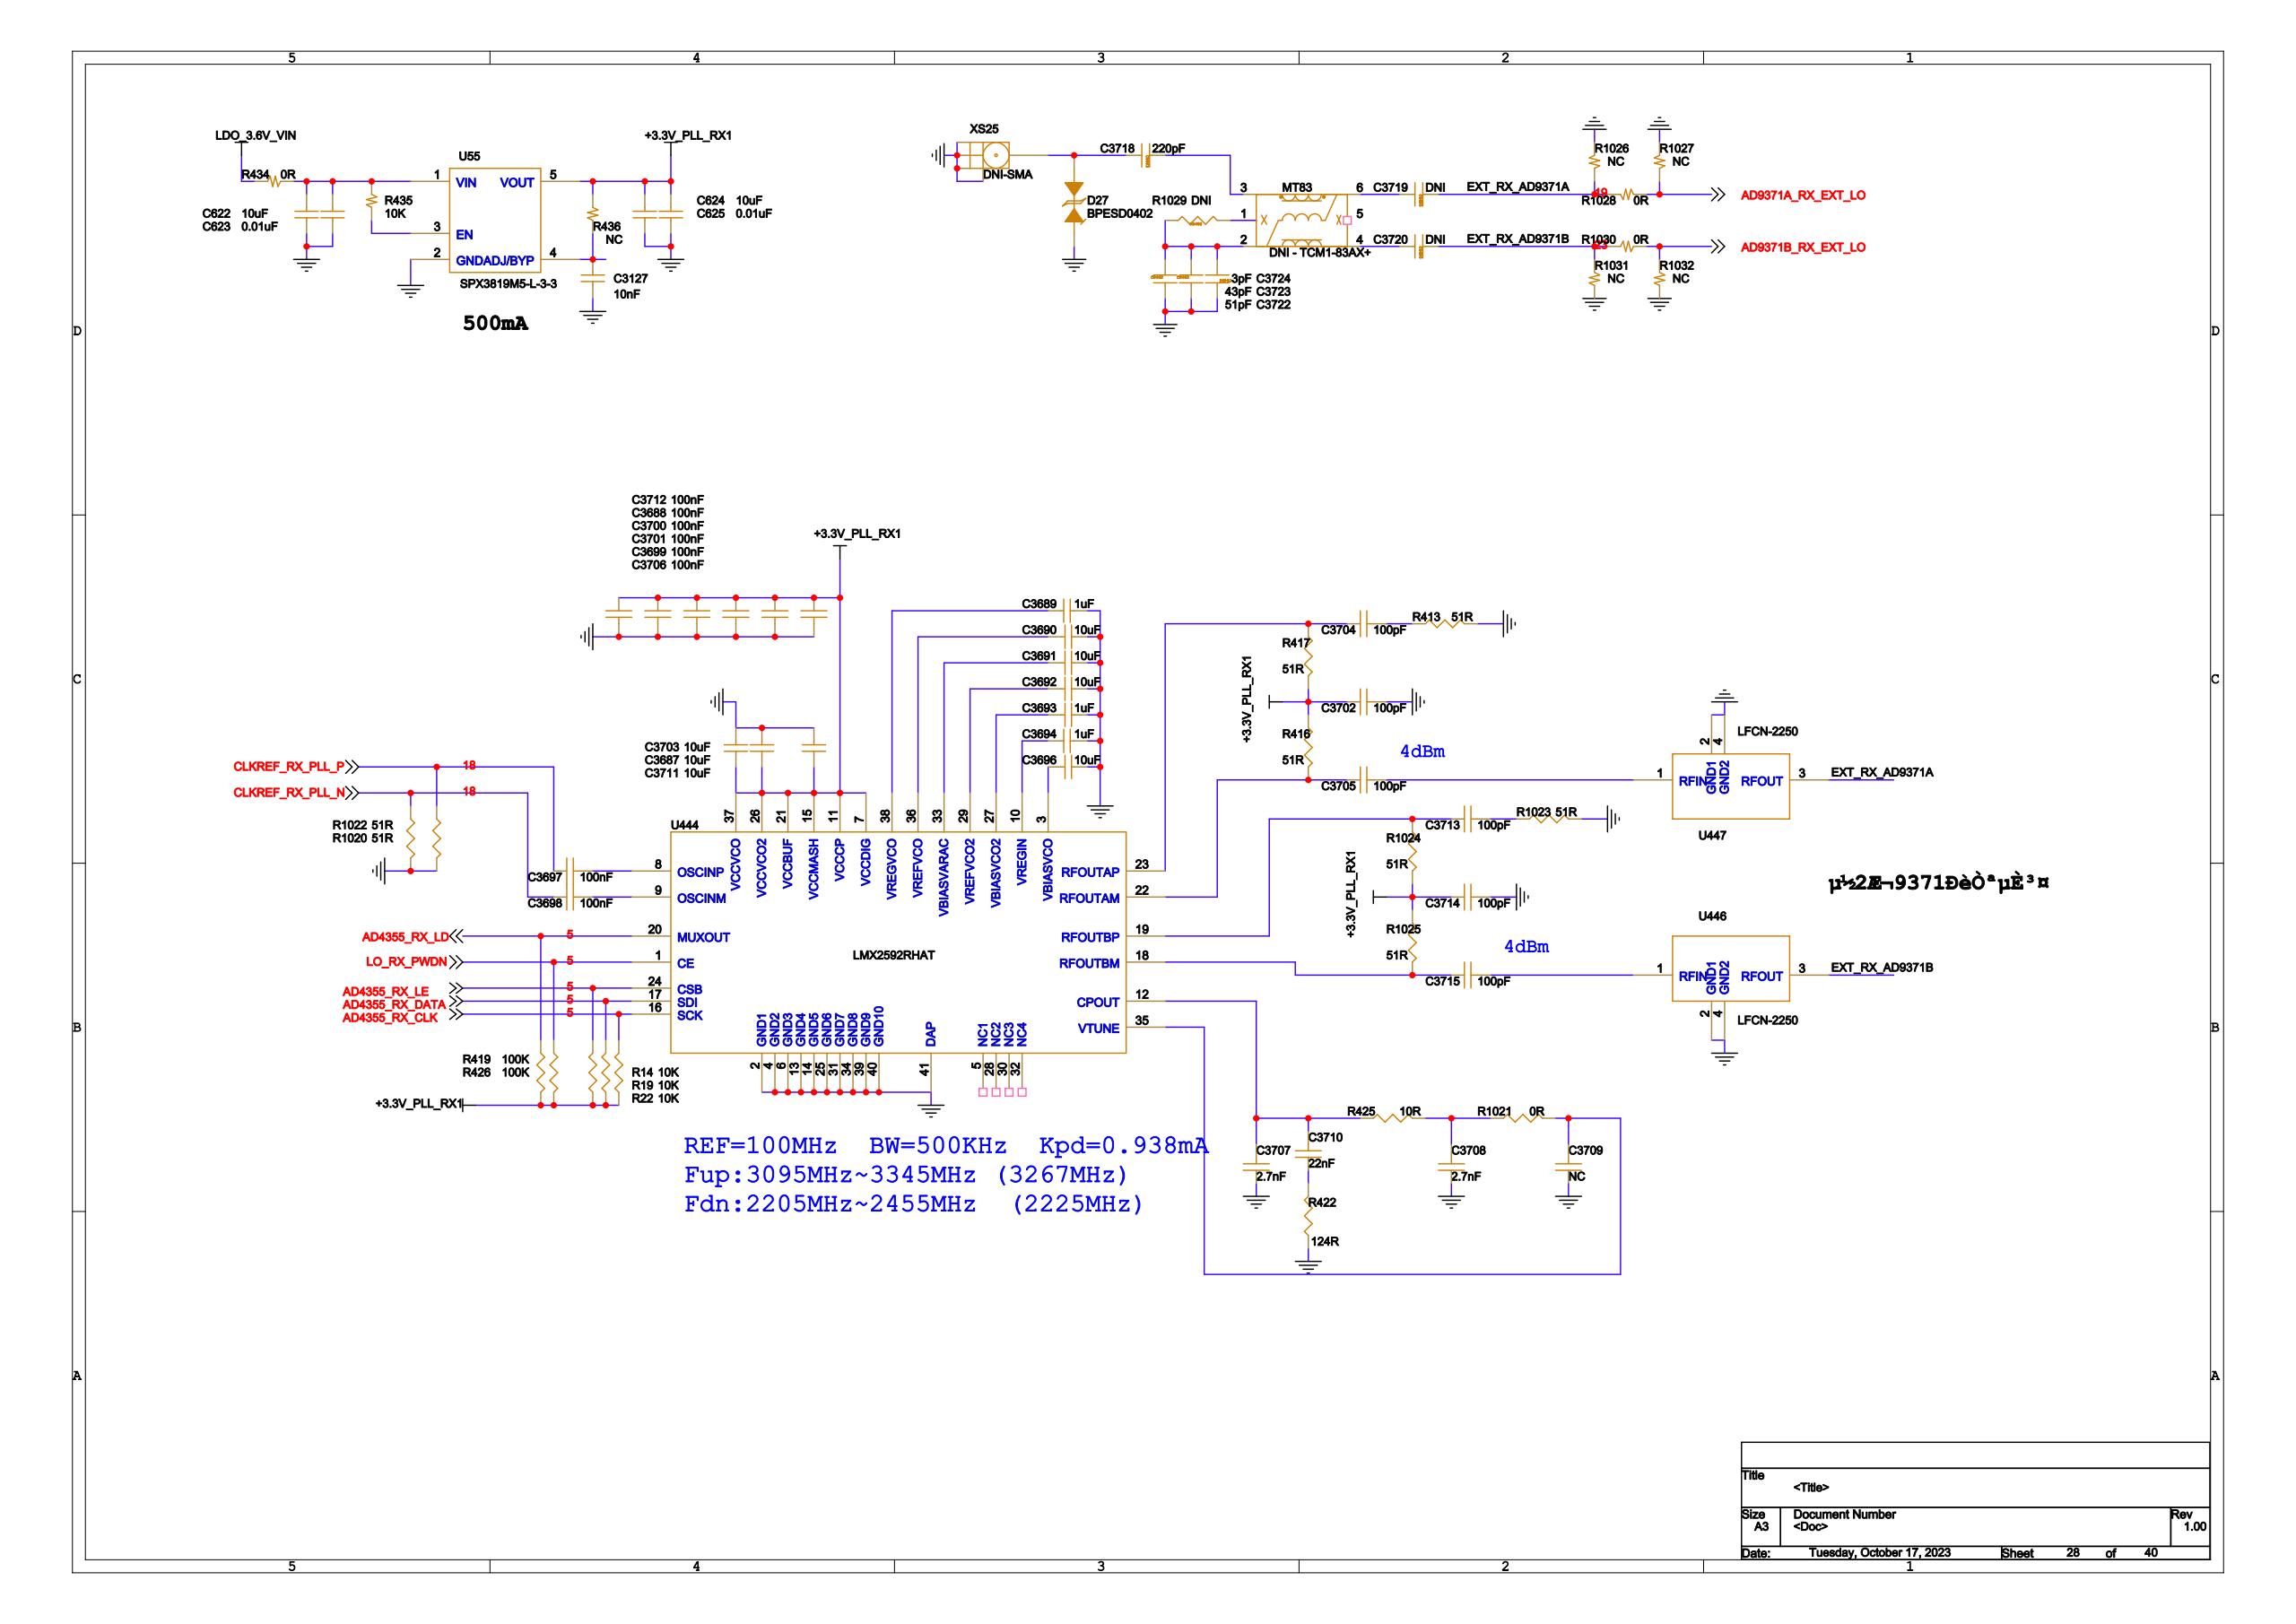Circuit board | Cadence Allegro | 1793 parts | 1223 nets | one sheet of the schematic
Parts on this sheet (reference | value | footprint):
C622 | 10uF | C0402
C623 | 0.01uF | C0402
C624 | 10uF | C0402
C625 | 0.01uF | C0402
C3127 | 10nF | C0402
C3687 | 10uF | C0402
C3688 | 100nF | C0402
C3689 | 1uF | C0402
C3690 | 10uF | C0402
C3691 | 10uF | C0402
C3692 | 10uF | C0402
C3693 | 1uF | C0402
C3694 | 1uF | C0402
C3696 | 10uF | C0402
C3697 | 100nF | C0402
C3698 | 100nF | C0402
C3699 | 100nF | C0402
C3700 | 100nF | C0402
C3701 | 100nF | C0402
C3702 | 100pF | C0402
C3703 | 10uF | C0402
C3704 | 100pF | C0402
C3705 | 100pF | C0402
C3706 | 100nF | C0402
C3707 | 2.7nF | C0402
C3708 | 2.7nF | C0402
C3709 | NC | C0402
C3710 | 22nF | C0402
C3711 | 10uF | C0402
C3712 | 100nF | C0402
C3713 | 100pF | C0402
C3714 | 100pF | C0402
C3715 | 100pF | C0402
C3718 | 220pF | C0402
C3719 | DNI | C0402
C3720 | DNI | C0402
C3722 | 51pF | C0402
C3723 | 43pF | C0402
C3724 | 3pF | C0402
D27 | BPESD0402 | C0402
MT83 | DNI - TCM1-83AX+ | TCM1-63AX
R14 | 10K | R0402
R19 | 10K | R0402
R22 | 10K | R0402
R413 | 51R | R0402
R416 | 51R | R0402
R417 | 51R | R0402
R419 | 100K | R0402
R422 | 124R | R0402
R425 | 10R | R0402
R426 | 100K | R0402
R434 | 0R | R0402
R435 | 10K | R0402
R436 | NC | R0402
R1020 | 51R | R0402
R1021 | 0R | R0402
R1022 | 51R | R0402
R1023 | 51R | R0402
R1024 | 51R | R0402
R1025 | 51R | R0402
R1026 | NC | R0402
R1027 | NC | R0402
R1028 | 0R | R0402
R1029 | DNI | R0402
R1030 | 0R | R0402
R1031 | NC | R0402
R1032 | NC | R0402
U55 | SPX3819M5-L-3-3 | SOT-23-5
U444 | LMX2592RHAT | QFN-41-050P600X600X100
U446 | LFCN-2250 | LFCN-3400
U447 | LFCN-2250 | LFCN-3400
XS25 | DNI-SMA | SMA_5X5MM
Nets of these parts (net: part-pin ...):
GND: C622-1 C623-1 C624-1 C625-1 C3127-2 C3687-2 C3688-2 C3689-2 C3690-1 C3691-1 C3692-1 C3693-1 C3694-2 C3696-1 C3699-2 C3700-2 C3701-2 C3702-2 C3703-2 C3706-2 C3707-1 C3708-1 C3709-1 C3711-2 C3712-2 C3714-2 C3722-2 C3723-2 C3724-1 D27-2 R413-1 R422-1 R1020-1 R1022-1 R1023-1 R1026-2 R1027-2 R1031-2 R1032-2 U55-2 U446-2 U446-4 U447-2 U447-4 XS25-2 XS25-3 XS25-4 XS25-5 U444-2 U444-4 U444-6 U444-13 U444-14 U444-25 U444-31 U444-34 U444-39 U444-40 U444-41
N17666070: C3718-2 D27-1 XS25-1
LDO_3.6V_VIN: R434-1
N17664931: C3715-2 U446-1
EXT_RX_AD9371B: C3720-1 R1030-1 R1031-1 U446-3
N17646626: C3705-2 U447-1
EXT_RX_AD9371A: C3719-1 R1026-1 R1028-1 U447-3
+3.3V_PLL_RX1: C624-2 C625-2 C3687-1 C3688-1 C3699-1 C3700-1 C3701-1 C3702-1 C3703-1 C3706-1 C3711-1 C3712-1 C3714-1 R14-1 R19-1 R22-1 R416-2 R417-1 R419-1 R426-1 R436-1 R1024-1 R1025-2 U55-5 U444-7 U444-11 U444-15 U444-21 U444-26 U444-37
N17646147: C3690-2 U444-36
N17646159: C3691-2 U444-33
N17646173: C3692-2 U444-29
N17646253: C3696-2 U444-3
N1566118: C622-2 C623-2 R434-2 R435-1 U55-1
N17646145: C3689-1 U444-38
N17646201: C3694-1 U444-10
N17646187: C3693-2 U444-27
N17666088: C3718-1 MT83-3
N17666102: C3719-2 MT83-6
N17666185: C3720-2 MT83-4
N17666142: MT83-1 R1029-1
N17666140: C3722-1 C3723-1 C3724-2 MT83-2 R1029-2
LO_RX_PWDN: R426-2 U444-1
N17646715: C3707-2 C3710-2 R425-1 U444-12
AD4355_RX_LE: R14-2 U444-24
AD4355_RX_LD: R419-2 U444-20
N17646364: C3698-2 U444-9
N17646344: C3697-2 U444-8
N17646107: C3705-1 R416-1 U444-22
N17646109: C3704-1 R417-2 U444-23
N17664866: C3713-1 R1024-2 U444-19
N17664927: C3715-1 R1025-1 U444-18
AD4355_RX_CLK: R22-2 U444-16
AD4355_RX_DATA: R19-2 U444-17
N17646749: C3709-2 R1021-2 U444-35
AD9371A_RX_EXT_LO: R1027-1 R1028-2
AD9371B_RX_EXT_LO: R1030-2 R1032-1
CLKREF_RX_PLL_P: C3697-1 R1020-2
CLKREF_RX_PLL_N: C3698-1 R1022-2
N17646624: C3704-2 R413-2
N17664870: C3713-2 R1023-2
N17646717: C3708-2 R425-2 R1021-1
N17646755: C3710-1 R422-2
N1566202: C3127-1 R436-2 U55-4
N1566390: R435-2 U55-3